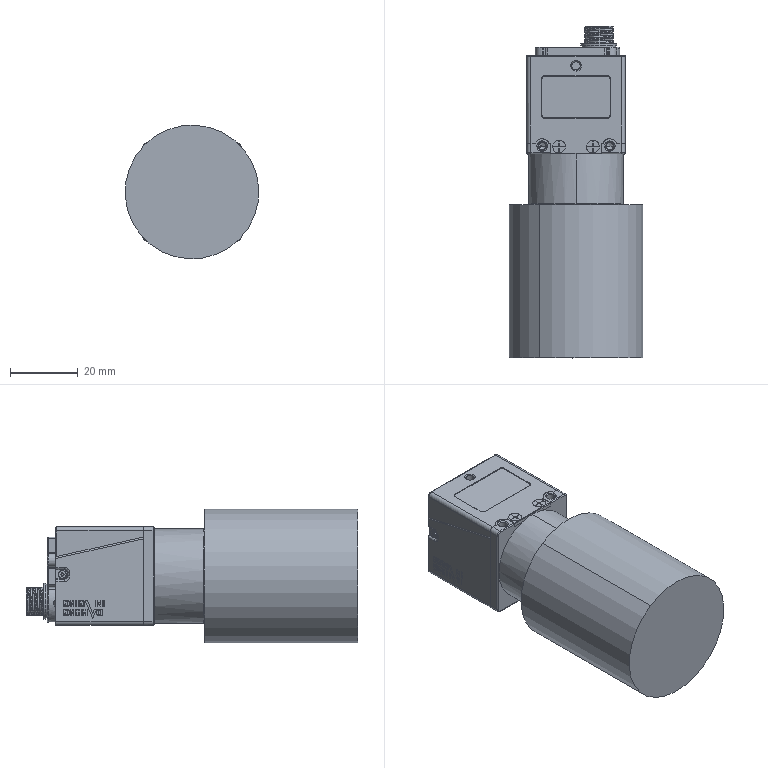Part | SolidWorks | 1 solid | 1436 faces | box 39.5 x 98.192 x 39.5 mm | volume 79084 mm3 | plane 776 | cylinder 384 | spline 170 | cone 103 | torus 3 | commonest cylinder face diameters 0.4 x84 1.4 x39 8.5 x21 2 x20 1 x17 0.6 x15